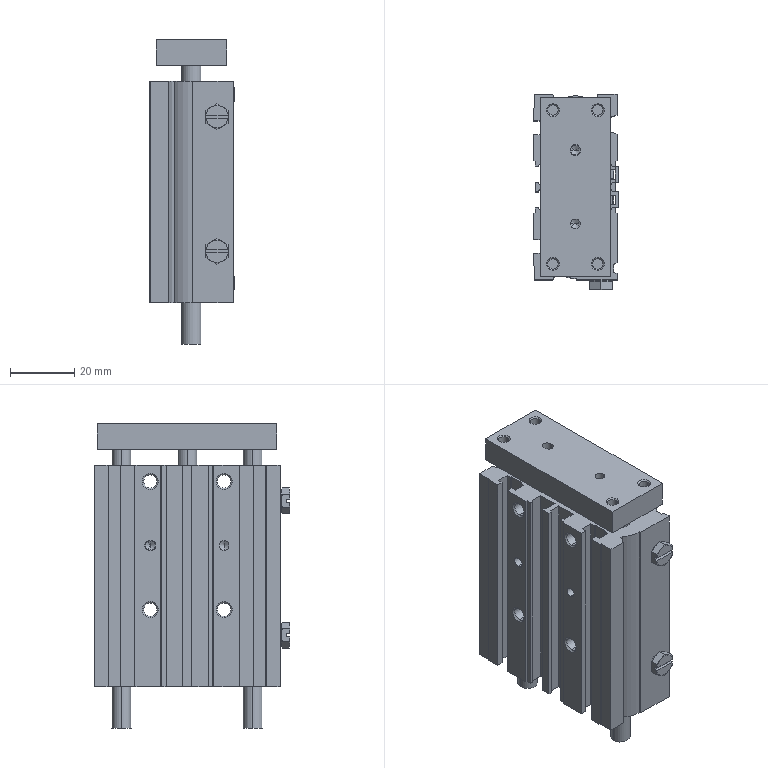Part | SolidWorks | 6 solids | 451 faces | box 26.4 x 61 x 95 mm | volume 91411 mm3 | plane 235 | cylinder 124 | cone 92 | commonest cylinder face diameters 3 x18 3.242 x16 4.134 x16 6 x16 0.8 x8 4.3 x8